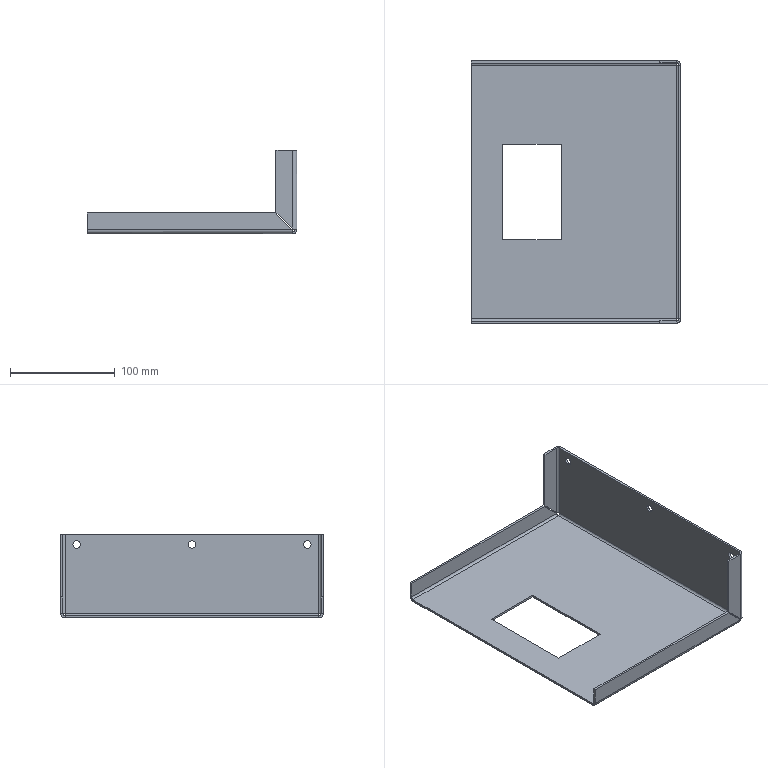Part | NX | features BREP 1 | 1 solid | 56 faces | box 200 x 250 x 80 mm | volume 144913 mm3 | plane 36 | cylinder 16 | spline 4 | commonest cylinder face diameters 7 x6 4 x5 8 x5